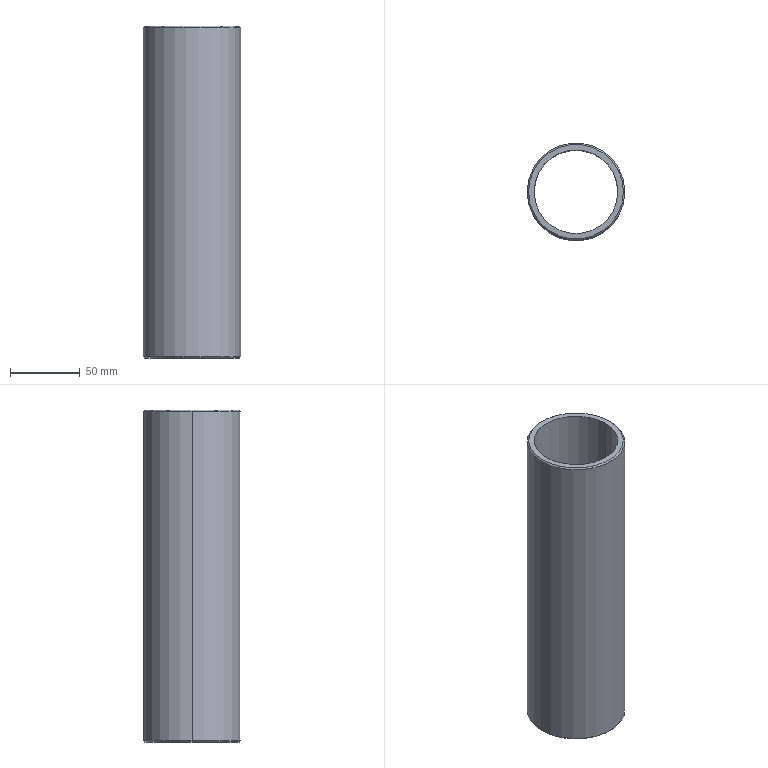Part | SolidWorks | features Chamfer 1, Extrusion 1 | 1 solid | 10 faces | box 70 x 70 x 238 mm | volume 242784 mm3 | cone 4 | cylinder 4 | plane 2 | commonest cylinder face diameters 60 x2 70 x2
STEP:
#1=CARTESIAN_POINT('',(34.,0.,238.));
#2=VERTEX_POINT('',#1);
#3=CARTESIAN_POINT('',(-34.,0.,238.));
#4=VERTEX_POINT('',#3);
#5=CARTESIAN_POINT('',(0.,0.,238.));
#6=DIRECTION('',(0.,0.,1.));
#7=DIRECTION('',(1.,0.,0.));
#8=AXIS2_PLACEMENT_3D('',#5,#6,#7);
#9=CIRCLE('',#8,34.);
#10=EDGE_CURVE('',#2,#4,#9,.T.);
#11=ORIENTED_EDGE('',*,*,#10,.F.);
#12=CARTESIAN_POINT('',(35.,0.,237.));
#13=VERTEX_POINT('',#12);
#14=CARTESIAN_POINT('',(34.,0.,238.));
#15=DIRECTION('',(0.7071,0.,-0.7071));
#16=VECTOR('',#15,1000.);
#17=LINE('',#14,#16);
#18=EDGE_CURVE('',#2,#13,#17,.T.);
#19=ORIENTED_EDGE('',*,*,#18,.T.);
#20=CARTESIAN_POINT('',(-35.,0.,237.));
#21=VERTEX_POINT('',#20);
#22=CARTESIAN_POINT('',(0.,0.,237.));
#23=DIRECTION('',(0.,0.,-1.));
#24=DIRECTION('',(1.,0.,0.));
#25=AXIS2_PLACEMENT_3D('',#22,#23,#24);
#26=CIRCLE('',#25,35.);
#27=EDGE_CURVE('',#21,#13,#26,.T.);
#28=ORIENTED_EDGE('',*,*,#27,.F.);
#29=CARTESIAN_POINT('',(-34.,0.,238.));
#30=DIRECTION('',(-0.7071,0.,-0.7071));
#31=VECTOR('',#30,1000.);
#32=LINE('',#29,#31);
#33=EDGE_CURVE('',#4,#21,#32,.T.);
#34=ORIENTED_EDGE('',*,*,#33,.F.);
#35=EDGE_LOOP('',(#11,#19,#28,#34));
#36=FACE_OUTER_BOUND('',#35,.T.);
#37=CARTESIAN_POINT('',(0.,0.,238.));
#38=DIRECTION('',(0.,0.,-1.));
#39=DIRECTION('',(-1.,0.,0.));
#40=AXIS2_PLACEMENT_3D('',#37,#38,#39);
#41=CONICAL_SURFACE('',#40,34.,0.7854);
#42=ADVANCED_FACE('',(#36),#41,.T.);
#43=CARTESIAN_POINT('',(-34.,0.,0.));
#44=VERTEX_POINT('',#43);
#45=CARTESIAN_POINT('',(34.,0.,0.));
#46=VERTEX_POINT('',#45);
#47=CARTESIAN_POINT('',(0.,0.,0.));
#48=DIRECTION('',(0.,0.,-1.));
#49=DIRECTION('',(1.,0.,0.));
#50=AXIS2_PLACEMENT_3D('',#47,#48,#49);
#51=CIRCLE('',#50,34.);
#52=EDGE_CURVE('',#44,#46,#51,.T.);
#53=ORIENTED_EDGE('',*,*,#52,.F.);
#54=CARTESIAN_POINT('',(-35.,0.,1.));
#55=VERTEX_POINT('',#54);
#56=CARTESIAN_POINT('',(-35.,0.,1.));
#57=DIRECTION('',(-0.7071,0.,0.7071));
#58=VECTOR('',#57,1000.);
#59=LINE('',#56,#58);
#60=EDGE_CURVE('',#44,#55,#59,.T.);
#61=ORIENTED_EDGE('',*,*,#60,.T.);
#62=CARTESIAN_POINT('',(35.,0.,1.));
#63=VERTEX_POINT('',#62);
#64=CARTESIAN_POINT('',(0.,0.,1.));
#65=DIRECTION('',(0.,0.,1.));
#66=DIRECTION('',(1.,0.,0.));
#67=AXIS2_PLACEMENT_3D('',#64,#65,#66);
#68=CIRCLE('',#67,35.);
#69=EDGE_CURVE('',#63,#55,#68,.T.);
#70=ORIENTED_EDGE('',*,*,#69,.F.);
#71=CARTESIAN_POINT('',(35.,0.,1.));
#72=DIRECTION('',(0.7071,0.,0.7071));
#73=VECTOR('',#72,1000.);
#74=LINE('',#71,#73);
#75=EDGE_CURVE('',#46,#63,#74,.T.);
#76=ORIENTED_EDGE('',*,*,#75,.F.);
#77=EDGE_LOOP('',(#53,#61,#70,#76));
#78=FACE_OUTER_BOUND('',#77,.T.);
#79=CARTESIAN_POINT('',(0.,0.,1.));
#80=DIRECTION('',(0.,0.,1.));
#81=DIRECTION('',(1.,0.,0.));
#82=AXIS2_PLACEMENT_3D('',#79,#80,#81);
#83=CONICAL_SURFACE('',#82,35.,0.7854);
#84=ADVANCED_FACE('',(#78),#83,.T.);
#85=CARTESIAN_POINT('',(-30.,0.,238.));
#86=VERTEX_POINT('',#85);
#87=CARTESIAN_POINT('',(30.,0.,238.));
#88=VERTEX_POINT('',#87);
#89=CARTESIAN_POINT('',(0.,0.,238.));
#90=DIRECTION('',(0.,0.,1.));
#91=DIRECTION('',(1.,0.,0.));
#92=AXIS2_PLACEMENT_3D('',#89,#90,#91);
#93=CIRCLE('',#92,30.);
#94=EDGE_CURVE('',#86,#88,#93,.T.);
#95=ORIENTED_EDGE('',*,*,#94,.T.);
#96=CARTESIAN_POINT('',(30.,0.,0.));
#97=VERTEX_POINT('',#96);
#98=CARTESIAN_POINT('',(30.,0.,238.));
#99=DIRECTION('',(0.,0.,-1.));
#100=VECTOR('',#99,1000.);
#101=LINE('',#98,#100);
#102=EDGE_CURVE('',#88,#97,#101,.T.);
#103=ORIENTED_EDGE('',*,*,#102,.T.);
#104=CARTESIAN_POINT('',(-30.,0.,0.));
#105=VERTEX_POINT('',#104);
#106=CARTESIAN_POINT('',(0.,0.,0.));
#107=DIRECTION('',(0.,0.,1.));
#108=DIRECTION('',(1.,0.,0.));
#109=AXIS2_PLACEMENT_3D('',#106,#107,#108);
#110=CIRCLE('',#109,30.);
#111=EDGE_CURVE('',#105,#97,#110,.T.);
#112=ORIENTED_EDGE('',*,*,#111,.F.);
#113=CARTESIAN_POINT('',(-30.,0.,238.));
#114=DIRECTION('',(0.,0.,-1.));
#115=VECTOR('',#114,1000.);
#116=LINE('',#113,#115);
#117=EDGE_CURVE('',#86,#105,#116,.T.);
#118=ORIENTED_EDGE('',*,*,#117,.F.);
#119=EDGE_LOOP('',(#95,#103,#112,#118));
#120=FACE_OUTER_BOUND('',#119,.T.);
#121=CARTESIAN_POINT('',(0.,0.,238.));
#122=DIRECTION('',(0.,0.,-1.));
#123=DIRECTION('',(-1.,0.,0.));
#124=AXIS2_PLACEMENT_3D('',#121,#122,#123);
#125=CYLINDRICAL_SURFACE('',#124,30.);
#126=ADVANCED_FACE('',(#120),#125,.F.);
#127=ORIENTED_EDGE('',*,*,#27,.T.);
#128=CARTESIAN_POINT('',(35.,0.,238.));
#129=DIRECTION('',(0.,0.,-1.));
#130=VECTOR('',#129,1000.);
#131=LINE('',#128,#130);
#132=EDGE_CURVE('',#13,#63,#131,.T.);
#133=ORIENTED_EDGE('',*,*,#132,.T.);
#134=ORIENTED_EDGE('',*,*,#69,.T.);
#135=CARTESIAN_POINT('',(-35.,0.,238.));
#136=DIRECTION('',(0.,0.,-1.));
#137=VECTOR('',#136,1000.);
#138=LINE('',#135,#137);
#139=EDGE_CURVE('',#21,#55,#138,.T.);
#140=ORIENTED_EDGE('',*,*,#139,.F.);
#141=EDGE_LOOP('',(#127,#133,#134,#140));
#142=FACE_OUTER_BOUND('',#141,.T.);
#143=CARTESIAN_POINT('',(0.,0.,238.));
#144=DIRECTION('',(0.,0.,-1.));
#145=DIRECTION('',(-1.,0.,0.));
#146=AXIS2_PLACEMENT_3D('',#143,#144,#145);
#147=CYLINDRICAL_SURFACE('',#146,35.);
#148=ADVANCED_FACE('',(#142),#147,.T.);
#149=CARTESIAN_POINT('',(0.,0.,238.));
#150=DIRECTION('',(0.,0.,1.));
#151=DIRECTION('',(1.,0.,0.));
#152=AXIS2_PLACEMENT_3D('',#149,#150,#151);
#153=CIRCLE('',#152,34.);
#154=EDGE_CURVE('',#4,#2,#153,.T.);
#155=ORIENTED_EDGE('',*,*,#154,.T.);
#156=ORIENTED_EDGE('',*,*,#10,.T.);
#157=EDGE_LOOP('',(#155,#156));
#158=FACE_OUTER_BOUND('',#157,.T.);
#159=ORIENTED_EDGE('',*,*,#94,.F.);
#160=CARTESIAN_POINT('',(0.,0.,238.));
#161=DIRECTION('',(0.,0.,1.));
#162=DIRECTION('',(1.,0.,0.));
#163=AXIS2_PLACEMENT_3D('',#160,#161,#162);
#164=CIRCLE('',#163,30.);
#165=EDGE_CURVE('',#88,#86,#164,.T.);
#166=ORIENTED_EDGE('',*,*,#165,.F.);
#167=EDGE_LOOP('',(#159,#166));
#168=FACE_BOUND('',#167,.T.);
#169=CARTESIAN_POINT('',(0.,0.,238.));
#170=DIRECTION('',(0.,0.,1.));
#171=DIRECTION('',(1.,0.,0.));
#172=AXIS2_PLACEMENT_3D('',#169,#170,#171);
#173=PLANE('',#172);
#174=ADVANCED_FACE('',(#158,#168),#173,.T.);
#175=CARTESIAN_POINT('',(0.,0.,0.));
#176=DIRECTION('',(0.,0.,-1.));
#177=DIRECTION('',(1.,0.,0.));
#178=AXIS2_PLACEMENT_3D('',#175,#176,#177);
#179=CIRCLE('',#178,34.);
#180=EDGE_CURVE('',#46,#44,#179,.T.);
#181=ORIENTED_EDGE('',*,*,#180,.T.);
#182=ORIENTED_EDGE('',*,*,#52,.T.);
#183=EDGE_LOOP('',(#181,#182));
#184=FACE_OUTER_BOUND('',#183,.T.);
#185=ORIENTED_EDGE('',*,*,#111,.T.);
#186=CARTESIAN_POINT('',(0.,0.,0.));
#187=DIRECTION('',(0.,0.,1.));
#188=DIRECTION('',(1.,0.,0.));
#189=AXIS2_PLACEMENT_3D('',#186,#187,#188);
#190=CIRCLE('',#189,30.);
#191=EDGE_CURVE('',#97,#105,#190,.T.);
#192=ORIENTED_EDGE('',*,*,#191,.T.);
#193=EDGE_LOOP('',(#185,#192));
#194=FACE_BOUND('',#193,.T.);
#195=CARTESIAN_POINT('',(0.,0.,0.));
#196=DIRECTION('',(0.,0.,1.));
#197=DIRECTION('',(1.,0.,0.));
#198=AXIS2_PLACEMENT_3D('',#195,#196,#197);
#199=PLANE('',#198);
#200=ADVANCED_FACE('',(#184,#194),#199,.F.);
#201=ORIENTED_EDGE('',*,*,#132,.F.);
#202=CARTESIAN_POINT('',(0.,0.,237.));
#203=DIRECTION('',(0.,0.,-1.));
#204=DIRECTION('',(1.,0.,0.));
#205=AXIS2_PLACEMENT_3D('',#202,#203,#204);
#206=CIRCLE('',#205,35.);
#207=EDGE_CURVE('',#13,#21,#206,.T.);
#208=ORIENTED_EDGE('',*,*,#207,.T.);
#209=ORIENTED_EDGE('',*,*,#139,.T.);
#210=CARTESIAN_POINT('',(0.,0.,1.));
#211=DIRECTION('',(0.,0.,1.));
#212=DIRECTION('',(1.,0.,0.));
#213=AXIS2_PLACEMENT_3D('',#210,#211,#212);
#214=CIRCLE('',#213,35.);
#215=EDGE_CURVE('',#55,#63,#214,.T.);
#216=ORIENTED_EDGE('',*,*,#215,.T.);
#217=EDGE_LOOP('',(#201,#208,#209,#216));
#218=FACE_OUTER_BOUND('',#217,.T.);
#219=CARTESIAN_POINT('',(0.,0.,238.));
#220=DIRECTION('',(0.,0.,-1.));
#221=DIRECTION('',(-1.,0.,0.));
#222=AXIS2_PLACEMENT_3D('',#219,#220,#221);
#223=CYLINDRICAL_SURFACE('',#222,35.);
#224=ADVANCED_FACE('',(#218),#223,.T.);
#225=ORIENTED_EDGE('',*,*,#102,.F.);
#226=ORIENTED_EDGE('',*,*,#165,.T.);
#227=ORIENTED_EDGE('',*,*,#117,.T.);
#228=ORIENTED_EDGE('',*,*,#191,.F.);
#229=EDGE_LOOP('',(#225,#226,#227,#228));
#230=FACE_OUTER_BOUND('',#229,.T.);
#231=CARTESIAN_POINT('',(0.,0.,238.));
#232=DIRECTION('',(0.,0.,-1.));
#233=DIRECTION('',(-1.,0.,0.));
#234=AXIS2_PLACEMENT_3D('',#231,#232,#233);
#235=CYLINDRICAL_SURFACE('',#234,30.);
#236=ADVANCED_FACE('',(#230),#235,.F.);
#237=ORIENTED_EDGE('',*,*,#60,.F.);
#238=ORIENTED_EDGE('',*,*,#180,.F.);
#239=ORIENTED_EDGE('',*,*,#75,.T.);
#240=ORIENTED_EDGE('',*,*,#215,.F.);
#241=EDGE_LOOP('',(#237,#238,#239,#240));
#242=FACE_OUTER_BOUND('',#241,.T.);
#243=CARTESIAN_POINT('',(0.,0.,1.));
#244=DIRECTION('',(0.,0.,1.));
#245=DIRECTION('',(1.,0.,0.));
#246=AXIS2_PLACEMENT_3D('',#243,#244,#245);
#247=CONICAL_SURFACE('',#246,35.,0.7854);
#248=ADVANCED_FACE('',(#242),#247,.T.);
#249=ORIENTED_EDGE('',*,*,#18,.F.);
#250=ORIENTED_EDGE('',*,*,#154,.F.);
#251=ORIENTED_EDGE('',*,*,#33,.T.);
#252=ORIENTED_EDGE('',*,*,#207,.F.);
#253=EDGE_LOOP('',(#249,#250,#251,#252));
#254=FACE_OUTER_BOUND('',#253,.T.);
#255=CARTESIAN_POINT('',(0.,0.,238.));
#256=DIRECTION('',(0.,0.,-1.));
#257=DIRECTION('',(-1.,0.,0.));
#258=AXIS2_PLACEMENT_3D('',#255,#256,#257);
#259=CONICAL_SURFACE('',#258,34.,0.7854);
#260=ADVANCED_FACE('',(#254),#259,.T.);
#261=CLOSED_SHELL('',(#42,#84,#126,#148,#174,#200,#224,#236,#248,#260));
#262=MANIFOLD_SOLID_BREP('',#261);
#263=CARTESIAN_POINT('',(0.,0.,0.));
#264=DIRECTION('',(0.,0.,1.));
#265=DIRECTION('',(1.,0.,0.));
#266=AXIS2_PLACEMENT_3D('',#263,#264,#265);
#267=(LENGTH_UNIT()NAMED_UNIT(*)SI_UNIT(.MILLI.,.METRE.));
#268=UNCERTAINTY_MEASURE_WITH_UNIT(LENGTH_MEASURE(0.00001),#267,'','');
#269=(NAMED_UNIT(*)PLANE_ANGLE_UNIT()SI_UNIT($,.RADIAN.));
#270=(NAMED_UNIT(*)SI_UNIT($,.STERADIAN.)SOLID_ANGLE_UNIT());
#271=(GEOMETRIC_REPRESENTATION_CONTEXT(3)GLOBAL_UNCERTAINTY_ASSIGNED_CONTEXT((#268))GLOBAL_UNIT_ASSIGNED_CONTEXT((#267,#269,#270))REPRESENTATION_CONTEXT('',''));
#272=ADVANCED_BREP_SHAPE_REPRESENTATION('',(#262,#266),#271);